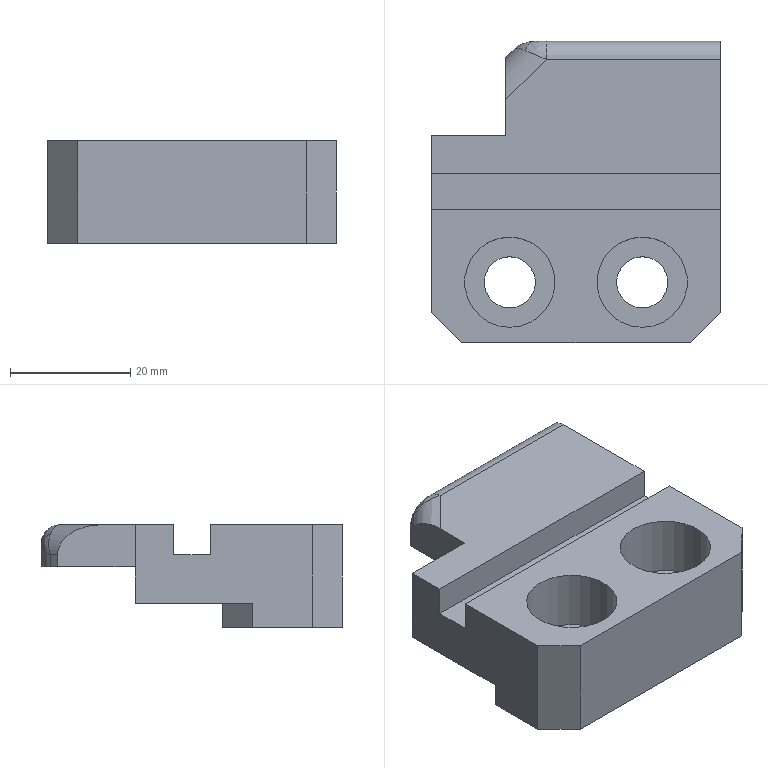Part | STEP file | gslz 2016.10.28-13_id314_x_t | 1 solid | 31 faces | box 48 x 50 x 17 mm | volume 22804 mm3 | plane 22 | cylinder 7 | spline 2 | commonest cylinder face diameters 8.5 x2 10 x2 15 x2 6 x1